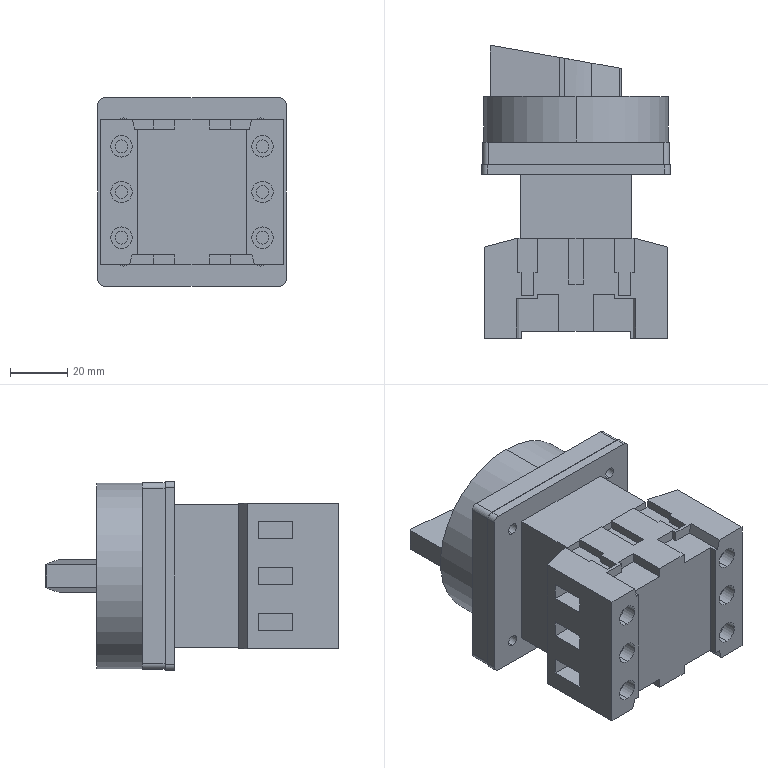Part | SolidWorks | features BaseBody 1 | 1 solid | 221 faces | box 66 x 102.704 x 66 mm | volume 215531 mm3 | plane 160 | cylinder 61 | commonest cylinder face diameters 4 x16 4.5 x12 7.5 x12 60 x8 63 x4 53 x3